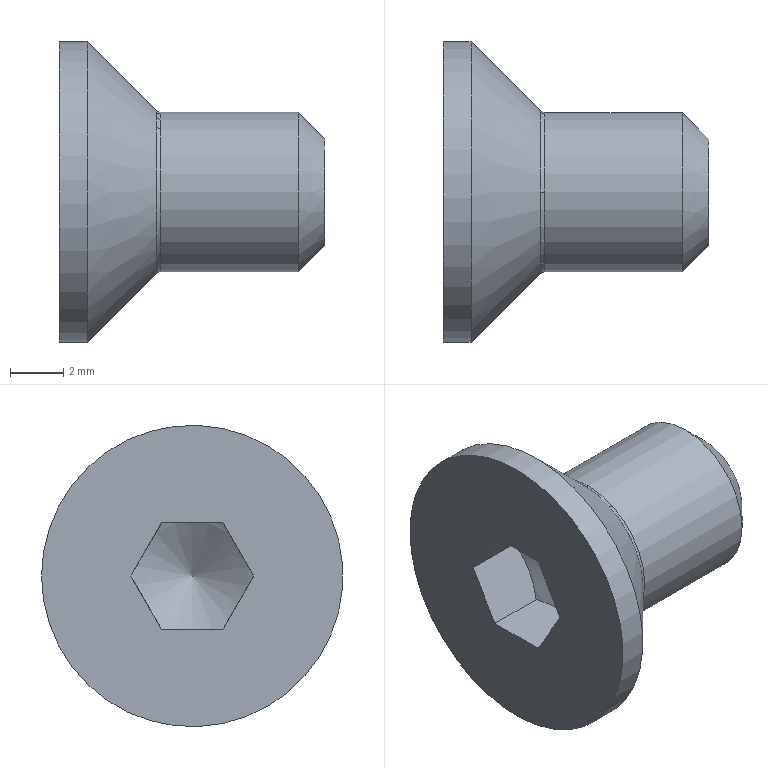Part | STEP file | Винт с потайной головкой и шестигранным углублением под ключ ГОСТ Р ИСО 10642 - М6 x 10 - 8.8 | 1 solid | 15 faces | box 10 x 11.34 x 11.34 mm | volume 400.146 mm3 | plane 8 | cone 3 | cylinder 2 | torus 2 | commonest cylinder face diameters 6 x1 11.34 x1
STEP:
#1=CARTESIAN_POINT('',(0.,5.67,0.));
#2=VERTEX_POINT('',#1);
#3=CARTESIAN_POINT('',(0.,0.,0.));
#4=DIRECTION('',(1.,0.,0.));
#5=DIRECTION('',(0.,1.,0.));
#6=AXIS2_PLACEMENT_3D('',#3,#4,#5);
#7=CIRCLE('',#6,5.67);
#8=EDGE_CURVE('',#2,#2,#7,.T.);
#9=ORIENTED_EDGE('',*,*,#8,.F.);
#10=EDGE_LOOP('',(#9));
#11=FACE_BOUND('',#10,.T.);
#12=CARTESIAN_POINT('',(0.,-1.155,2.));
#13=VERTEX_POINT('',#12);
#14=CARTESIAN_POINT('',(0.,-2.309,0.));
#15=VERTEX_POINT('',#14);
#16=CARTESIAN_POINT('',(0.,-1.155,2.));
#17=DIRECTION('',(0.,-0.5,-0.866));
#18=VECTOR('',#17,1.);
#19=LINE('',#16,#18);
#20=EDGE_CURVE('',#13,#15,#19,.T.);
#21=ORIENTED_EDGE('',*,*,#20,.T.);
#22=CARTESIAN_POINT('',(0.,-1.155,-2.));
#23=VERTEX_POINT('',#22);
#24=CARTESIAN_POINT('',(0.,-2.309,0.));
#25=DIRECTION('',(0.,0.5,-0.866));
#26=VECTOR('',#25,1.);
#27=LINE('',#24,#26);
#28=EDGE_CURVE('',#15,#23,#27,.T.);
#29=ORIENTED_EDGE('',*,*,#28,.T.);
#30=CARTESIAN_POINT('',(0.,1.155,-2.));
#31=VERTEX_POINT('',#30);
#32=CARTESIAN_POINT('',(0.,-1.155,-2.));
#33=DIRECTION('',(0.,1.,0.));
#34=VECTOR('',#33,1.);
#35=LINE('',#32,#34);
#36=EDGE_CURVE('',#23,#31,#35,.T.);
#37=ORIENTED_EDGE('',*,*,#36,.T.);
#38=CARTESIAN_POINT('',(0.,2.309,0.));
#39=VERTEX_POINT('',#38);
#40=CARTESIAN_POINT('',(0.,1.155,-2.));
#41=DIRECTION('',(0.,0.5,0.866));
#42=VECTOR('',#41,1.);
#43=LINE('',#40,#42);
#44=EDGE_CURVE('',#31,#39,#43,.T.);
#45=ORIENTED_EDGE('',*,*,#44,.T.);
#46=CARTESIAN_POINT('',(0.,1.155,2.));
#47=VERTEX_POINT('',#46);
#48=CARTESIAN_POINT('',(0.,2.309,0.));
#49=DIRECTION('',(0.,-0.5,0.866));
#50=VECTOR('',#49,1.);
#51=LINE('',#48,#50);
#52=EDGE_CURVE('',#39,#47,#51,.T.);
#53=ORIENTED_EDGE('',*,*,#52,.T.);
#54=CARTESIAN_POINT('',(0.,1.155,2.));
#55=DIRECTION('',(0.,-1.,0.));
#56=VECTOR('',#55,1.);
#57=LINE('',#54,#56);
#58=EDGE_CURVE('',#47,#13,#57,.T.);
#59=ORIENTED_EDGE('',*,*,#58,.T.);
#60=EDGE_LOOP('',(#21,#29,#37,#45,#53,#59));
#61=FACE_BOUND('',#60,.T.);
#62=CARTESIAN_POINT('',(0.,0.,0.));
#63=DIRECTION('',(1.,0.,0.));
#64=DIRECTION('',(0.,0.,1.));
#65=AXIS2_PLACEMENT_3D('',#62,#63,#64);
#66=PLANE('',#65);
#67=ADVANCED_FACE('',(#11,#61),#66,.F.);
#68=CARTESIAN_POINT('',(2.2,1.155,2.));
#69=VERTEX_POINT('',#68);
#70=CARTESIAN_POINT('',(2.379,0.,2.));
#71=VERTEX_POINT('',#70);
#72=CARTESIAN_POINT('',(2.379,0.,2.));
#73=CARTESIAN_POINT('',(2.379,0.03993,2.));
#74=CARTESIAN_POINT('',(2.378,0.09305,2.));
#75=CARTESIAN_POINT('',(2.374,0.1977,2.));
#76=CARTESIAN_POINT('',(2.367,0.2984,2.));
#77=CARTESIAN_POINT('',(2.356,0.3998,2.));
#78=CARTESIAN_POINT('',(2.342,0.5139,2.));
#79=CARTESIAN_POINT('',(2.325,0.6191,2.));
#80=CARTESIAN_POINT('',(2.301,0.7452,2.));
#81=CARTESIAN_POINT('',(2.279,0.8524,2.));
#82=CARTESIAN_POINT('',(2.256,0.9483,2.));
#83=CARTESIAN_POINT('',(2.232,1.04,2.));
#84=CARTESIAN_POINT('',(2.216,1.1,2.));
#85=CARTESIAN_POINT('',(2.203,1.143,2.));
#86=CARTESIAN_POINT('',(2.2,1.155,2.));
#87=B_SPLINE_CURVE_WITH_KNOTS('',3,(#72,#73,#74,#75,#76,#77,#78,#79,#80,#81,#82,#83,#84,#85,#86),.UNSPECIFIED.,.F.,.F.,(4,1,1,1,1,1,1,1,1,1,1,1,4),(0.,0.1021,0.1359,0.2681,0.3604,0.3966,0.5625,0.6326,0.7252,0.8429,0.8848,0.9686,1.),.UNSPECIFIED.);
#88=EDGE_CURVE('',#69,#71,#87,.F.);
#89=ORIENTED_EDGE('',*,*,#88,.F.);
#90=CARTESIAN_POINT('',(2.2,2.309,0.));
#91=VERTEX_POINT('',#90);
#92=CARTESIAN_POINT('',(2.2,1.155,2.));
#93=CARTESIAN_POINT('',(2.204,1.162,1.987));
#94=CARTESIAN_POINT('',(2.212,1.176,1.962));
#95=CARTESIAN_POINT('',(2.225,1.198,1.924));
#96=CARTESIAN_POINT('',(2.236,1.22,1.886));
#97=CARTESIAN_POINT('',(2.248,1.242,1.848));
#98=CARTESIAN_POINT('',(2.259,1.264,1.81));
#99=CARTESIAN_POINT('',(2.269,1.287,1.771));
#100=CARTESIAN_POINT('',(2.28,1.309,1.733));
#101=CARTESIAN_POINT('',(2.29,1.332,1.694));
#102=CARTESIAN_POINT('',(2.3,1.355,1.652));
#103=CARTESIAN_POINT('',(2.31,1.381,1.607));
#104=CARTESIAN_POINT('',(2.322,1.415,1.549));
#105=CARTESIAN_POINT('',(2.337,1.46,1.472));
#106=CARTESIAN_POINT('',(2.352,1.514,1.378));
#107=CARTESIAN_POINT('',(2.364,1.568,1.283));
#108=CARTESIAN_POINT('',(2.371,1.614,1.205));
#109=CARTESIAN_POINT('',(2.375,1.65,1.143));
#110=CARTESIAN_POINT('',(2.377,1.681,1.088));
#111=CARTESIAN_POINT('',(2.378,1.709,1.04));
#112=CARTESIAN_POINT('',(2.379,1.731,1.002));
#113=CARTESIAN_POINT('',(2.379,1.753,0.9644));
#114=CARTESIAN_POINT('',(2.378,1.78,0.9178));
#115=CARTESIAN_POINT('',(2.375,1.813,0.8602));
#116=CARTESIAN_POINT('',(2.371,1.846,0.8026));
#117=CARTESIAN_POINT('',(2.366,1.879,0.7449));
#118=CARTESIAN_POINT('',(2.36,1.913,0.6872));
#119=CARTESIAN_POINT('',(2.353,1.946,0.6295));
#120=CARTESIAN_POINT('',(2.344,1.979,0.5718));
#121=CARTESIAN_POINT('',(2.334,2.013,0.5142));
#122=CARTESIAN_POINT('',(2.323,2.046,0.4566));
#123=CARTESIAN_POINT('',(2.311,2.079,0.3992));
#124=CARTESIAN_POINT('',(2.298,2.112,0.3418));
#125=CARTESIAN_POINT('',(2.284,2.145,0.2846));
#126=CARTESIAN_POINT('',(2.269,2.178,0.2274));
#127=CARTESIAN_POINT('',(2.253,2.211,0.1704));
#128=CARTESIAN_POINT('',(2.236,2.244,0.1134));
#129=CARTESIAN_POINT('',(2.219,2.277,0.05661));
#130=CARTESIAN_POINT('',(2.206,2.299,0.01885));
#131=CARTESIAN_POINT('',(2.2,2.309,0.));
#132=B_SPLINE_CURVE_WITH_KNOTS('',3,(#92,#93,#94,#95,#96,#97,#98,#99,#100,#101,#102,#103,#104,#105,#106,#107,#108,#109,#110,#111,#112,#113,#114,#115,#116,#117,#118,#119,#120,#121,#122,#123,#124,#125,#126,#127,#128,#129,#130,#131),.UNSPECIFIED.,.F.,.F.,(4,1,1,1,1,1,1,1,1,1,1,1,1,1,1,1,1,1,1,1,1,1,1,1,1,1,1,1,1,1,1,1,1,1,1,1,1,4),(0.,0.01933,0.03868,0.05804,0.07746,0.0969,0.1164,0.136,0.1557,0.1754,0.1981,0.2236,0.2627,0.3137,0.3641,0.403,0.4296,0.4566,0.4843,0.5,0.5121,0.5404,0.5688,0.5973,0.6258,0.6543,0.6829,0.7116,0.7402,0.7689,0.7977,0.8264,0.8552,0.8841,0.913,0.9419,0.9709,1.),.UNSPECIFIED.);
#133=EDGE_CURVE('',#91,#69,#132,.F.);
#134=ORIENTED_EDGE('',*,*,#133,.F.);
#135=CARTESIAN_POINT('',(2.2,1.155,-2.));
#136=VERTEX_POINT('',#135);
#137=CARTESIAN_POINT('',(2.2,2.309,0.));
#138=CARTESIAN_POINT('',(2.204,2.302,-0.01256));
#139=CARTESIAN_POINT('',(2.212,2.288,-0.03772));
#140=CARTESIAN_POINT('',(2.225,2.266,-0.07557));
#141=CARTESIAN_POINT('',(2.236,2.244,-0.1136));
#142=CARTESIAN_POINT('',(2.248,2.222,-0.1517));
#143=CARTESIAN_POINT('',(2.259,2.2,-0.1901));
#144=CARTESIAN_POINT('',(2.269,2.177,-0.2286));
#145=CARTESIAN_POINT('',(2.28,2.155,-0.2674));
#146=CARTESIAN_POINT('',(2.29,2.132,-0.3065));
#147=CARTESIAN_POINT('',(2.3,2.109,-0.3476));
#148=CARTESIAN_POINT('',(2.31,2.083,-0.3926));
#149=CARTESIAN_POINT('',(2.322,2.049,-0.4507));
#150=CARTESIAN_POINT('',(2.337,2.005,-0.528));
#151=CARTESIAN_POINT('',(2.352,1.95,-0.6222));
#152=CARTESIAN_POINT('',(2.364,1.896,-0.7166));
#153=CARTESIAN_POINT('',(2.371,1.85,-0.7949));
#154=CARTESIAN_POINT('',(2.375,1.814,-0.8574));
#155=CARTESIAN_POINT('',(2.377,1.783,-0.9124));
#156=CARTESIAN_POINT('',(2.378,1.755,-0.96));
#157=CARTESIAN_POINT('',(2.379,1.733,-0.9976));
#158=CARTESIAN_POINT('',(2.379,1.711,-1.036));
#159=CARTESIAN_POINT('',(2.378,1.685,-1.082));
#160=CARTESIAN_POINT('',(2.375,1.651,-1.14));
#161=CARTESIAN_POINT('',(2.371,1.618,-1.197));
#162=CARTESIAN_POINT('',(2.366,1.585,-1.255));
#163=CARTESIAN_POINT('',(2.36,1.551,-1.313));
#164=CARTESIAN_POINT('',(2.353,1.518,-1.371));
#165=CARTESIAN_POINT('',(2.344,1.485,-1.428));
#166=CARTESIAN_POINT('',(2.334,1.452,-1.486));
#167=CARTESIAN_POINT('',(2.323,1.418,-1.543));
#168=CARTESIAN_POINT('',(2.311,1.385,-1.601));
#169=CARTESIAN_POINT('',(2.298,1.352,-1.658));
#170=CARTESIAN_POINT('',(2.284,1.319,-1.715));
#171=CARTESIAN_POINT('',(2.269,1.286,-1.773));
#172=CARTESIAN_POINT('',(2.253,1.253,-1.83));
#173=CARTESIAN_POINT('',(2.236,1.22,-1.887));
#174=CARTESIAN_POINT('',(2.219,1.187,-1.943));
#175=CARTESIAN_POINT('',(2.206,1.166,-1.981));
#176=CARTESIAN_POINT('',(2.2,1.155,-2.));
#177=B_SPLINE_CURVE_WITH_KNOTS('',3,(#137,#138,#139,#140,#141,#142,#143,#144,#145,#146,#147,#148,#149,#150,#151,#152,#153,#154,#155,#156,#157,#158,#159,#160,#161,#162,#163,#164,#165,#166,#167,#168,#169,#170,#171,#172,#173,#174,#175,#176),.UNSPECIFIED.,.F.,.F.,(4,1,1,1,1,1,1,1,1,1,1,1,1,1,1,1,1,1,1,1,1,1,1,1,1,1,1,1,1,1,1,1,1,1,1,1,1,4),(0.,0.01933,0.03868,0.05804,0.07746,0.0969,0.1164,0.136,0.1557,0.1754,0.1981,0.2236,0.2627,0.3137,0.3641,0.403,0.4296,0.4566,0.4843,0.5,0.5121,0.5404,0.5688,0.5973,0.6258,0.6543,0.6829,0.7116,0.7402,0.7689,0.7977,0.8264,0.8552,0.8841,0.913,0.9419,0.9709,1.),.UNSPECIFIED.);
#178=EDGE_CURVE('',#136,#91,#177,.F.);
#179=ORIENTED_EDGE('',*,*,#178,.F.);
#180=CARTESIAN_POINT('',(2.2,-1.155,-2.));
#181=VERTEX_POINT('',#180);
#182=CARTESIAN_POINT('',(2.2,1.155,-2.));
#183=CARTESIAN_POINT('',(2.204,1.14,-2.));
#184=CARTESIAN_POINT('',(2.212,1.111,-2.));
#185=CARTESIAN_POINT('',(2.225,1.067,-2.));
#186=CARTESIAN_POINT('',(2.236,1.026,-2.));
#187=CARTESIAN_POINT('',(2.243,0.9963,-2.));
#188=CARTESIAN_POINT('',(2.251,0.9668,-2.));
#189=CARTESIAN_POINT('',(2.259,0.9352,-2.));
#190=CARTESIAN_POINT('',(2.269,0.8907,-2.));
#191=CARTESIAN_POINT('',(2.28,0.8459,-2.));
#192=CARTESIAN_POINT('',(2.29,0.8008,-2.));
#193=CARTESIAN_POINT('',(2.3,0.7534,-2.));
#194=CARTESIAN_POINT('',(2.31,0.7013,-2.));
#195=CARTESIAN_POINT('',(2.317,0.6639,-2.));
#196=CARTESIAN_POINT('',(2.326,0.6142,-2.));
#197=CARTESIAN_POINT('',(2.337,0.5447,-2.));
#198=CARTESIAN_POINT('',(2.349,0.4569,-2.));
#199=CARTESIAN_POINT('',(2.358,0.3781,-2.));
#200=CARTESIAN_POINT('',(2.365,0.3087,-2.));
#201=CARTESIAN_POINT('',(2.37,0.2457,-2.));
#202=CARTESIAN_POINT('',(2.373,0.1946,-2.));
#203=CARTESIAN_POINT('',(2.375,0.1527,-2.));
#204=CARTESIAN_POINT('',(2.377,0.1011,-2.));
#205=CARTESIAN_POINT('',(2.378,0.04616,-2.));
#206=CARTESIAN_POINT('',(2.379,0.002789,-2.));
#207=CARTESIAN_POINT('',(2.379,-0.04112,-2.));
#208=CARTESIAN_POINT('',(2.378,-0.07585,-2.));
#209=CARTESIAN_POINT('',(2.377,-0.1201,-2.));
#210=CARTESIAN_POINT('',(2.375,-0.1645,-2.));
#211=CARTESIAN_POINT('',(2.371,-0.228,-2.));
#212=CARTESIAN_POINT('',(2.366,-0.2946,-2.));
#213=CARTESIAN_POINT('',(2.361,-0.3498,-2.));
#214=CARTESIAN_POINT('',(2.356,-0.3942,-2.));
#215=CARTESIAN_POINT('',(2.351,-0.4386,-2.));
#216=CARTESIAN_POINT('',(2.344,-0.4944,-2.));
#217=CARTESIAN_POINT('',(2.335,-0.5545,-2.));
#218=CARTESIAN_POINT('',(2.328,-0.5988,-2.));
#219=CARTESIAN_POINT('',(2.32,-0.6431,-2.));
#220=CARTESIAN_POINT('',(2.311,-0.6938,-2.));
#221=CARTESIAN_POINT('',(2.298,-0.76,-2.));
#222=CARTESIAN_POINT('',(2.285,-0.8199,-2.));
#223=CARTESIAN_POINT('',(2.276,-0.8639,-2.));
#224=CARTESIAN_POINT('',(2.265,-0.9079,-2.));
#225=CARTESIAN_POINT('',(2.253,-0.958,-2.));
#226=CARTESIAN_POINT('',(2.237,-1.023,-2.));
#227=CARTESIAN_POINT('',(2.225,-1.066,-2.));
#228=CARTESIAN_POINT('',(2.213,-1.11,-2.));
#229=CARTESIAN_POINT('',(2.206,-1.133,-2.));
#230=CARTESIAN_POINT('',(2.2,-1.155,-2.));
#231=B_SPLINE_CURVE_WITH_KNOTS('',3,(#182,#183,#184,#185,#186,#187,#188,#189,#190,#191,#192,#193,#194,#195,#196,#197,#198,#199,#200,#201,#202,#203,#204,#205,#206,#207,#208,#209,#210,#211,#212,#213,#214,#215,#216,#217,#218,#219,#220,#221,#222,#223,#224,#225,#226,#227,#228,#229,#230),.UNSPECIFIED.,.F.,.F.,(4,1,1,1,1,1,1,1,1,1,1,1,1,1,1,1,1,1,1,1,1,1,1,1,1,1,1,1,1,1,1,1,1,1,1,1,1,1,1,1,1,1,1,1,1,1,4),(0.,0.01933,0.03868,0.05804,0.07472,0.07746,0.0969,0.1164,0.136,0.1557,0.1754,0.1981,0.2236,0.2241,0.2627,0.3137,0.3375,0.3641,0.403,0.4183,0.4296,0.4566,0.4843,0.5,0.5121,0.5404,0.5444,0.5688,0.5973,0.6258,0.6543,0.6683,0.6829,0.7116,0.7402,0.7605,0.7689,0.7977,0.8264,0.8552,0.876,0.8841,0.913,0.9419,0.9694,0.9709,1.),.UNSPECIFIED.);
#232=EDGE_CURVE('',#181,#136,#231,.F.);
#233=ORIENTED_EDGE('',*,*,#232,.F.);
#234=CARTESIAN_POINT('',(2.2,-2.309,0.));
#235=VERTEX_POINT('',#234);
#236=CARTESIAN_POINT('',(2.2,-1.155,-2.));
#237=CARTESIAN_POINT('',(2.204,-1.162,-1.987));
#238=CARTESIAN_POINT('',(2.212,-1.176,-1.962));
#239=CARTESIAN_POINT('',(2.225,-1.198,-1.924));
#240=CARTESIAN_POINT('',(2.236,-1.22,-1.886));
#241=CARTESIAN_POINT('',(2.248,-1.242,-1.848));
#242=CARTESIAN_POINT('',(2.259,-1.264,-1.81));
#243=CARTESIAN_POINT('',(2.269,-1.287,-1.771));
#244=CARTESIAN_POINT('',(2.28,-1.309,-1.733));
#245=CARTESIAN_POINT('',(2.29,-1.332,-1.694));
#246=CARTESIAN_POINT('',(2.3,-1.355,-1.652));
#247=CARTESIAN_POINT('',(2.31,-1.381,-1.607));
#248=CARTESIAN_POINT('',(2.322,-1.415,-1.549));
#249=CARTESIAN_POINT('',(2.337,-1.459,-1.472));
#250=CARTESIAN_POINT('',(2.352,-1.514,-1.378));
#251=CARTESIAN_POINT('',(2.364,-1.568,-1.284));
#252=CARTESIAN_POINT('',(2.371,-1.613,-1.206));
#253=CARTESIAN_POINT('',(2.375,-1.649,-1.144));
#254=CARTESIAN_POINT('',(2.377,-1.681,-1.089));
#255=CARTESIAN_POINT('',(2.378,-1.708,-1.041));
#256=CARTESIAN_POINT('',(2.379,-1.73,-1.003));
#257=CARTESIAN_POINT('',(2.379,-1.752,-0.9655));
#258=CARTESIAN_POINT('',(2.378,-1.779,-0.9195));
#259=CARTESIAN_POINT('',(2.375,-1.812,-0.862));
#260=CARTESIAN_POINT('',(2.372,-1.845,-0.8045));
#261=CARTESIAN_POINT('',(2.367,-1.878,-0.7468));
#262=CARTESIAN_POINT('',(2.36,-1.912,-0.6892));
#263=CARTESIAN_POINT('',(2.353,-1.945,-0.6314));
#264=CARTESIAN_POINT('',(2.344,-1.978,-0.5737));
#265=CARTESIAN_POINT('',(2.335,-2.011,-0.516));
#266=CARTESIAN_POINT('',(2.324,-2.045,-0.4583));
#267=CARTESIAN_POINT('',(2.312,-2.078,-0.4007));
#268=CARTESIAN_POINT('',(2.299,-2.111,-0.3432));
#269=CARTESIAN_POINT('',(2.284,-2.144,-0.2857));
#270=CARTESIAN_POINT('',(2.269,-2.178,-0.2284));
#271=CARTESIAN_POINT('',(2.253,-2.211,-0.1711));
#272=CARTESIAN_POINT('',(2.236,-2.244,-0.1139));
#273=CARTESIAN_POINT('',(2.219,-2.277,-0.05687));
#274=CARTESIAN_POINT('',(2.206,-2.298,-0.01894));
#275=CARTESIAN_POINT('',(2.2,-2.309,0.));
#276=B_SPLINE_CURVE_WITH_KNOTS('',3,(#236,#237,#238,#239,#240,#241,#242,#243,#244,#245,#246,#247,#248,#249,#250,#251,#252,#253,#254,#255,#256,#257,#258,#259,#260,#261,#262,#263,#264,#265,#266,#267,#268,#269,#270,#271,#272,#273,#274,#275),.UNSPECIFIED.,.F.,.F.,(4,1,1,1,1,1,1,1,1,1,1,1,1,1,1,1,1,1,1,1,1,1,1,1,1,1,1,1,1,1,1,1,1,1,1,1,1,4),(0.,0.01933,0.03868,0.05804,0.07746,0.0969,0.1164,0.136,0.1557,0.1754,0.198,0.2236,0.2626,0.3135,0.3638,0.4026,0.4291,0.456,0.4836,0.5,0.5114,0.5396,0.5679,0.5963,0.6248,0.6533,0.6819,0.7106,0.7393,0.7681,0.7969,0.8257,0.8546,0.8836,0.9126,0.9417,0.9708,1.),.UNSPECIFIED.);
#277=EDGE_CURVE('',#235,#181,#276,.F.);
#278=ORIENTED_EDGE('',*,*,#277,.F.);
#279=CARTESIAN_POINT('',(2.2,-1.155,2.));
#280=VERTEX_POINT('',#279);
#281=CARTESIAN_POINT('',(2.2,-2.309,0.));
#282=CARTESIAN_POINT('',(2.204,-2.302,0.01256));
#283=CARTESIAN_POINT('',(2.212,-2.288,0.03772));
#284=CARTESIAN_POINT('',(2.225,-2.266,0.07557));
#285=CARTESIAN_POINT('',(2.236,-2.244,0.1136));
#286=CARTESIAN_POINT('',(2.248,-2.222,0.1517));
#287=CARTESIAN_POINT('',(2.259,-2.2,0.1901));
#288=CARTESIAN_POINT('',(2.269,-2.177,0.2286));
#289=CARTESIAN_POINT('',(2.28,-2.155,0.2674));
#290=CARTESIAN_POINT('',(2.29,-2.132,0.3065));
#291=CARTESIAN_POINT('',(2.3,-2.109,0.3476));
#292=CARTESIAN_POINT('',(2.31,-2.083,0.3926));
#293=CARTESIAN_POINT('',(2.322,-2.049,0.4507));
#294=CARTESIAN_POINT('',(2.337,-2.005,0.528));
#295=CARTESIAN_POINT('',(2.352,-1.95,0.6222));
#296=CARTESIAN_POINT('',(2.364,-1.896,0.7166));
#297=CARTESIAN_POINT('',(2.371,-1.85,0.7949));
#298=CARTESIAN_POINT('',(2.375,-1.814,0.8574));
#299=CARTESIAN_POINT('',(2.377,-1.783,0.9124));
#300=CARTESIAN_POINT('',(2.378,-1.755,0.96));
#301=CARTESIAN_POINT('',(2.379,-1.733,0.9976));
#302=CARTESIAN_POINT('',(2.379,-1.711,1.036));
#303=CARTESIAN_POINT('',(2.378,-1.685,1.082));
#304=CARTESIAN_POINT('',(2.375,-1.651,1.14));
#305=CARTESIAN_POINT('',(2.371,-1.618,1.197));
#306=CARTESIAN_POINT('',(2.366,-1.585,1.255));
#307=CARTESIAN_POINT('',(2.36,-1.551,1.313));
#308=CARTESIAN_POINT('',(2.353,-1.518,1.371));
#309=CARTESIAN_POINT('',(2.344,-1.485,1.428));
#310=CARTESIAN_POINT('',(2.334,-1.452,1.486));
#311=CARTESIAN_POINT('',(2.323,-1.418,1.543));
#312=CARTESIAN_POINT('',(2.311,-1.385,1.601));
#313=CARTESIAN_POINT('',(2.298,-1.352,1.658));
#314=CARTESIAN_POINT('',(2.284,-1.319,1.715));
#315=CARTESIAN_POINT('',(2.269,-1.286,1.773));
#316=CARTESIAN_POINT('',(2.253,-1.253,1.83));
#317=CARTESIAN_POINT('',(2.236,-1.22,1.887));
#318=CARTESIAN_POINT('',(2.219,-1.187,1.943));
#319=CARTESIAN_POINT('',(2.206,-1.166,1.981));
#320=CARTESIAN_POINT('',(2.2,-1.155,2.));
#321=B_SPLINE_CURVE_WITH_KNOTS('',3,(#281,#282,#283,#284,#285,#286,#287,#288,#289,#290,#291,#292,#293,#294,#295,#296,#297,#298,#299,#300,#301,#302,#303,#304,#305,#306,#307,#308,#309,#310,#311,#312,#313,#314,#315,#316,#317,#318,#319,#320),.UNSPECIFIED.,.F.,.F.,(4,1,1,1,1,1,1,1,1,1,1,1,1,1,1,1,1,1,1,1,1,1,1,1,1,1,1,1,1,1,1,1,1,1,1,1,1,4),(0.,0.01933,0.03868,0.05804,0.07746,0.0969,0.1164,0.136,0.1557,0.1754,0.1981,0.2236,0.2627,0.3137,0.3641,0.403,0.4296,0.4566,0.4843,0.5,0.5121,0.5404,0.5688,0.5973,0.6258,0.6543,0.6829,0.7116,0.7402,0.7689,0.7977,0.8264,0.8552,0.8841,0.913,0.9419,0.9709,1.),.UNSPECIFIED.);
#322=EDGE_CURVE('',#280,#235,#321,.F.);
#323=ORIENTED_EDGE('',*,*,#322,.F.);
#324=CARTESIAN_POINT('',(2.2,-1.155,2.));
#325=CARTESIAN_POINT('',(2.208,-1.128,2.));
#326=CARTESIAN_POINT('',(2.224,-1.07,2.));
#327=CARTESIAN_POINT('',(2.246,-0.9856,2.));
#328=CARTESIAN_POINT('',(2.27,-0.8898,2.));
#329=CARTESIAN_POINT('',(2.291,-0.7956,2.));
#330=CARTESIAN_POINT('',(2.311,-0.698,2.));
#331=CARTESIAN_POINT('',(2.33,-0.5909,2.));
#332=CARTESIAN_POINT('',(2.342,-0.5072,2.));
#333=CARTESIAN_POINT('',(2.355,-0.4061,2.));
#334=CARTESIAN_POINT('',(2.365,-0.3138,2.));
#335=CARTESIAN_POINT('',(2.372,-0.2169,2.));
#336=CARTESIAN_POINT('',(2.377,-0.121,2.));
#337=CARTESIAN_POINT('',(2.379,-0.05776,2.));
#338=CARTESIAN_POINT('',(2.379,-0.005712,2.));
#339=CARTESIAN_POINT('',(2.379,-0.000000001,2.));
#340=B_SPLINE_CURVE_WITH_KNOTS('',3,(#324,#325,#326,#327,#328,#329,#330,#331,#332,#333,#334,#335,#336,#337,#338,#339),.UNSPECIFIED.,.F.,.F.,(4,1,1,1,1,1,1,1,1,1,1,1,1,4),(0.,0.07,0.1546,0.224,0.3223,0.4019,0.4787,0.6006,0.6184,0.7397,0.8381,0.8669,0.9854,1.),.UNSPECIFIED.);
#341=EDGE_CURVE('',#71,#280,#340,.F.);
#342=ORIENTED_EDGE('',*,*,#341,.F.);
#343=EDGE_LOOP('',(#89,#134,#179,#233,#278,#323,#342));
#344=FACE_BOUND('',#343,.T.);
#345=CARTESIAN_POINT('',(2.867,0.,0.));
#346=DIRECTION('',(-1.,0.,0.));
#347=DIRECTION('',(0.,0.,-1.));
#348=AXIS2_PLACEMENT_3D('',#345,#346,#347);
#349=CONICAL_SURFACE('',#348,1.155,1.047);
#350=ADVANCED_FACE('',(#344),#349,.F.);
#351=ORIENTED_EDGE('',*,*,#341,.T.);
#352=CARTESIAN_POINT('',(0.,-1.155,2.));
#353=DIRECTION('',(1.,0.,0.));
#354=VECTOR('',#353,1.);
#355=LINE('',#352,#354);
#356=EDGE_CURVE('',#13,#280,#355,.T.);
#357=ORIENTED_EDGE('',*,*,#356,.F.);
#358=ORIENTED_EDGE('',*,*,#58,.F.);
#359=CARTESIAN_POINT('',(0.,1.155,2.));
#360=DIRECTION('',(1.,0.,0.));
#361=VECTOR('',#360,1.);
#362=LINE('',#359,#361);
#363=EDGE_CURVE('',#47,#69,#362,.T.);
#364=ORIENTED_EDGE('',*,*,#363,.T.);
#365=ORIENTED_EDGE('',*,*,#88,.T.);
#366=EDGE_LOOP('',(#351,#357,#358,#364,#365));
#367=FACE_BOUND('',#366,.T.);
#368=CARTESIAN_POINT('',(0.,1.155,2.));
#369=DIRECTION('',(0.,0.,1.));
#370=DIRECTION('',(0.,-1.,0.));
#371=AXIS2_PLACEMENT_3D('',#368,#369,#370);
#372=PLANE('',#371);
#373=ADVANCED_FACE('',(#367),#372,.F.);
#374=ORIENTED_EDGE('',*,*,#133,.T.);
#375=ORIENTED_EDGE('',*,*,#363,.F.);
#376=ORIENTED_EDGE('',*,*,#52,.F.);
#377=CARTESIAN_POINT('',(0.,2.309,0.));
#378=DIRECTION('',(1.,0.,0.));
#379=VECTOR('',#378,1.);
#380=LINE('',#377,#379);
#381=EDGE_CURVE('',#39,#91,#380,.T.);
#382=ORIENTED_EDGE('',*,*,#381,.T.);
#383=EDGE_LOOP('',(#374,#375,#376,#382));
#384=FACE_BOUND('',#383,.T.);
#385=CARTESIAN_POINT('',(0.,2.309,0.));
#386=DIRECTION('',(0.,0.866,0.5));
#387=DIRECTION('',(0.,-0.5,0.866));
#388=AXIS2_PLACEMENT_3D('',#385,#386,#387);
#389=PLANE('',#388);
#390=ADVANCED_FACE('',(#384),#389,.F.);
#391=ORIENTED_EDGE('',*,*,#178,.T.);
#392=ORIENTED_EDGE('',*,*,#381,.F.);
#393=ORIENTED_EDGE('',*,*,#44,.F.);
#394=CARTESIAN_POINT('',(0.,1.155,-2.));
#395=DIRECTION('',(1.,0.,0.));
#396=VECTOR('',#395,1.);
#397=LINE('',#394,#396);
#398=EDGE_CURVE('',#31,#136,#397,.T.);
#399=ORIENTED_EDGE('',*,*,#398,.T.);
#400=EDGE_LOOP('',(#391,#392,#393,#399));
#401=FACE_BOUND('',#400,.T.);
#402=CARTESIAN_POINT('',(0.,1.155,-2.));
#403=DIRECTION('',(0.,0.866,-0.5));
#404=DIRECTION('',(0.,0.5,0.866));
#405=AXIS2_PLACEMENT_3D('',#402,#403,#404);
#406=PLANE('',#405);
#407=ADVANCED_FACE('',(#401),#406,.F.);
#408=ORIENTED_EDGE('',*,*,#232,.T.);
#409=ORIENTED_EDGE('',*,*,#398,.F.);
#410=ORIENTED_EDGE('',*,*,#36,.F.);
#411=CARTESIAN_POINT('',(0.,-1.155,-2.));
#412=DIRECTION('',(1.,0.,0.));
#413=VECTOR('',#412,1.);
#414=LINE('',#411,#413);
#415=EDGE_CURVE('',#23,#181,#414,.T.);
#416=ORIENTED_EDGE('',*,*,#415,.T.);
#417=EDGE_LOOP('',(#408,#409,#410,#416));
#418=FACE_BOUND('',#417,.T.);
#419=CARTESIAN_POINT('',(0.,-1.155,-2.));
#420=DIRECTION('',(0.,0.,-1.));
#421=DIRECTION('',(0.,1.,0.));
#422=AXIS2_PLACEMENT_3D('',#419,#420,#421);
#423=PLANE('',#422);
#424=ADVANCED_FACE('',(#418),#423,.F.);
#425=ORIENTED_EDGE('',*,*,#277,.T.);
#426=ORIENTED_EDGE('',*,*,#415,.F.);
#427=ORIENTED_EDGE('',*,*,#28,.F.);
#428=CARTESIAN_POINT('',(0.,-2.309,0.));
#429=DIRECTION('',(1.,0.,0.));
#430=VECTOR('',#429,1.);
#431=LINE('',#428,#430);
#432=EDGE_CURVE('',#15,#235,#431,.T.);
#433=ORIENTED_EDGE('',*,*,#432,.T.);
#434=EDGE_LOOP('',(#425,#426,#427,#433));
#435=FACE_BOUND('',#434,.T.);
#436=CARTESIAN_POINT('',(0.,-2.309,0.));
#437=DIRECTION('',(0.,-0.866,-0.5));
#438=DIRECTION('',(0.,0.5,-0.866));
#439=AXIS2_PLACEMENT_3D('',#436,#437,#438);
#440=PLANE('',#439);
#441=ADVANCED_FACE('',(#435),#440,.F.);
#442=ORIENTED_EDGE('',*,*,#322,.T.);
#443=ORIENTED_EDGE('',*,*,#432,.F.);
#444=ORIENTED_EDGE('',*,*,#20,.F.);
#445=ORIENTED_EDGE('',*,*,#356,.T.);
#446=EDGE_LOOP('',(#442,#443,#444,#445));
#447=FACE_BOUND('',#446,.T.);
#448=CARTESIAN_POINT('',(0.,-1.155,2.));
#449=DIRECTION('',(0.,-0.866,0.5));
#450=DIRECTION('',(0.,-0.5,-0.866));
#451=AXIS2_PLACEMENT_3D('',#448,#449,#450);
#452=PLANE('',#451);
#453=ADVANCED_FACE('',(#447),#452,.F.);
#454=CARTESIAN_POINT('',(1.05,5.67,0.));
#455=VERTEX_POINT('',#454);
#456=CARTESIAN_POINT('',(1.05,0.,0.));
#457=DIRECTION('',(1.,0.,0.));
#458=DIRECTION('',(0.,1.,0.));
#459=AXIS2_PLACEMENT_3D('',#456,#457,#458);
#460=CIRCLE('',#459,5.67);
#461=EDGE_CURVE('',#455,#455,#460,.T.);
#462=ORIENTED_EDGE('',*,*,#461,.F.);
#463=EDGE_LOOP('',(#462));
#464=FACE_OUTER_BOUND('',#463,.T.);
#465=ORIENTED_EDGE('',*,*,#8,.T.);
#466=EDGE_LOOP('',(#465));
#467=FACE_OUTER_BOUND('',#466,.T.);
#468=CARTESIAN_POINT('',(0.,0.,0.));
#469=DIRECTION('',(1.,0.,0.));
#470=DIRECTION('',(0.,1.,0.));
#471=AXIS2_PLACEMENT_3D('',#468,#469,#470);
#472=CYLINDRICAL_SURFACE('',#471,5.67);
#473=ADVANCED_FACE('',(#464,#467),#472,.T.);
#474=CARTESIAN_POINT('',(3.647,3.073,0.));
#475=VERTEX_POINT('',#474);
#476=CARTESIAN_POINT('',(3.647,0.,3.073));
#477=VERTEX_POINT('',#476);
#478=CARTESIAN_POINT('',(3.647,0.,0.));
#479=DIRECTION('',(1.,0.,0.));
#480=DIRECTION('',(0.,0.,1.));
#481=AXIS2_PLACEMENT_3D('',#478,#479,#480);
#482=CIRCLE('',#481,3.073);
#483=EDGE_CURVE('',#475,#477,#482,.F.);
#484=ORIENTED_EDGE('',*,*,#483,.T.);
#485=CARTESIAN_POINT('',(3.647,0.,0.));
#486=DIRECTION('',(1.,0.,0.));
#487=DIRECTION('',(0.,1.,0.));
#488=AXIS2_PLACEMENT_3D('',#485,#486,#487);
#489=CIRCLE('',#488,3.073);
#490=EDGE_CURVE('',#477,#475,#489,.F.);
#491=ORIENTED_EDGE('',*,*,#490,.T.);
#492=EDGE_LOOP('',(#484,#491));
#493=FACE_BOUND('',#492,.T.);
#494=ORIENTED_EDGE('',*,*,#461,.T.);
#495=EDGE_LOOP('',(#494));
#496=FACE_OUTER_BOUND('',#495,.T.);
#497=CARTESIAN_POINT('',(2.348,0.,0.));
#498=DIRECTION('',(-1.,0.,0.));
#499=DIRECTION('',(0.,-1.,0.));
#500=AXIS2_PLACEMENT_3D('',#497,#498,#499);
#501=CONICAL_SURFACE('',#500,4.372,0.7854);
#502=ADVANCED_FACE('',(#493,#496),#501,.T.);
#503=CARTESIAN_POINT('',(3.824,0.,3.));
#504=VERTEX_POINT('',#503);
#505=CARTESIAN_POINT('',(3.824,3.,0.));
#506=VERTEX_POINT('',#505);
#507=CARTESIAN_POINT('',(3.824,0.,0.));
#508=DIRECTION('',(1.,0.,0.));
#509=DIRECTION('',(0.,1.,0.));
#510=AXIS2_PLACEMENT_3D('',#507,#508,#509);
#511=CIRCLE('',#510,3.);
#512=EDGE_CURVE('',#504,#506,#511,.F.);
#513=ORIENTED_EDGE('',*,*,#512,.T.);
#514=CARTESIAN_POINT('',(3.824,3.25,0.));
#515=DIRECTION('',(0.,0.,-1.));
#516=DIRECTION('',(0.,-1.,0.));
#517=AXIS2_PLACEMENT_3D('',#514,#515,#516);
#518=CIRCLE('',#517,0.25);
#519=EDGE_CURVE('',#506,#475,#518,.T.);
#520=ORIENTED_EDGE('',*,*,#519,.T.);
#521=ORIENTED_EDGE('',*,*,#490,.F.);
#522=CARTESIAN_POINT('',(3.824,0.,3.25));
#523=DIRECTION('',(0.,1.,0.));
#524=DIRECTION('',(0.,0.,-1.));
#525=AXIS2_PLACEMENT_3D('',#522,#523,#524);
#526=CIRCLE('',#525,0.25);
#527=EDGE_CURVE('',#504,#477,#526,.T.);
#528=ORIENTED_EDGE('',*,*,#527,.F.);
#529=EDGE_LOOP('',(#513,#520,#521,#528));
#530=FACE_BOUND('',#529,.T.);
#531=CARTESIAN_POINT('',(3.824,0.,0.));
#532=DIRECTION('',(1.,0.,0.));
#533=DIRECTION('',(0.,0.9861,-0.1659));
#534=AXIS2_PLACEMENT_3D('',#531,#532,#533);
#535=TOROIDAL_SURFACE('',#534,3.25,0.25);
#536=ADVANCED_FACE('',(#530),#535,.F.);
#537=CARTESIAN_POINT('',(3.824,0.,0.));
#538=DIRECTION('',(1.,0.,0.));
#539=DIRECTION('',(0.,0.,1.));
#540=AXIS2_PLACEMENT_3D('',#537,#538,#539);
#541=CIRCLE('',#540,3.);
#542=EDGE_CURVE('',#506,#504,#541,.F.);
#543=ORIENTED_EDGE('',*,*,#542,.T.);
#544=ORIENTED_EDGE('',*,*,#527,.T.);
#545=ORIENTED_EDGE('',*,*,#483,.F.);
#546=ORIENTED_EDGE('',*,*,#519,.F.);
#547=EDGE_LOOP('',(#543,#544,#545,#546));
#548=FACE_BOUND('',#547,.T.);
#549=CARTESIAN_POINT('',(3.824,0.,0.));
#550=DIRECTION('',(1.,0.,0.));
#551=DIRECTION('',(0.,0.1659,0.9861));
#552=AXIS2_PLACEMENT_3D('',#549,#550,#551);
#553=TOROIDAL_SURFACE('',#552,3.25,0.25);
#554=ADVANCED_FACE('',(#548),#553,.F.);
#555=CARTESIAN_POINT('',(9.,0.,3.));
#556=VERTEX_POINT('',#555);
#557=CARTESIAN_POINT('',(9.,0.,0.));
#558=DIRECTION('',(1.,0.,0.));
#559=DIRECTION('',(0.,0.,1.));
#560=AXIS2_PLACEMENT_3D('',#557,#558,#559);
#561=CIRCLE('',#560,3.);
#562=EDGE_CURVE('',#556,#556,#561,.T.);
#563=ORIENTED_EDGE('',*,*,#562,.F.);
#564=EDGE_LOOP('',(#563));
#565=FACE_OUTER_BOUND('',#564,.T.);
#566=ORIENTED_EDGE('',*,*,#512,.F.);
#567=ORIENTED_EDGE('',*,*,#542,.F.);
#568=EDGE_LOOP('',(#566,#567));
#569=FACE_BOUND('',#568,.T.);
#570=CARTESIAN_POINT('',(0.,0.,0.));
#571=DIRECTION('',(1.,0.,0.));
#572=DIRECTION('',(0.,0.,1.));
#573=AXIS2_PLACEMENT_3D('',#570,#571,#572);
#574=CYLINDRICAL_SURFACE('',#573,3.);
#575=ADVANCED_FACE('',(#565,#569),#574,.T.);
#576=CARTESIAN_POINT('',(10.,0.,2.));
#577=VERTEX_POINT('',#576);
#578=CARTESIAN_POINT('',(10.,0.,0.));
#579=DIRECTION('',(1.,0.,0.));
#580=DIRECTION('',(0.,0.,1.));
#581=AXIS2_PLACEMENT_3D('',#578,#579,#580);
#582=CIRCLE('',#581,2.);
#583=EDGE_CURVE('',#577,#577,#582,.T.);
#584=ORIENTED_EDGE('',*,*,#583,.F.);
#585=EDGE_LOOP('',(#584));
#586=FACE_OUTER_BOUND('',#585,.T.);
#587=ORIENTED_EDGE('',*,*,#562,.T.);
#588=EDGE_LOOP('',(#587));
#589=FACE_OUTER_BOUND('',#588,.T.);
#590=CARTESIAN_POINT('',(9.5,0.,0.));
#591=DIRECTION('',(-1.,0.,0.));
#592=DIRECTION('',(0.,0.,-1.));
#593=AXIS2_PLACEMENT_3D('',#590,#591,#592);
#594=CONICAL_SURFACE('',#593,2.5,0.7854);
#595=ADVANCED_FACE('',(#586,#589),#594,.T.);
#596=ORIENTED_EDGE('',*,*,#583,.T.);
#597=EDGE_LOOP('',(#596));
#598=FACE_BOUND('',#597,.T.);
#599=CARTESIAN_POINT('',(10.,0.,0.));
#600=DIRECTION('',(1.,0.,0.));
#601=DIRECTION('',(0.,0.,1.));
#602=AXIS2_PLACEMENT_3D('',#599,#600,#601);
#603=PLANE('',#602);
#604=ADVANCED_FACE('',(#598),#603,.T.);
#605=CLOSED_SHELL('',(#67,#350,#373,#390,#407,#424,#441,#453,#473,#502,#536,#554,#575,#595,#604));
#606=MANIFOLD_SOLID_BREP('',#605);
#607=(LENGTH_UNIT()NAMED_UNIT(*)SI_UNIT(.MILLI.,.METRE.));
#608=UNCERTAINTY_MEASURE_WITH_UNIT(LENGTH_MEASURE(0.00001),#607,'','');
#609=(NAMED_UNIT(*)PLANE_ANGLE_UNIT()SI_UNIT($,.RADIAN.));
#610=(NAMED_UNIT(*)SI_UNIT($,.STERADIAN.)SOLID_ANGLE_UNIT());
#611=(GEOMETRIC_REPRESENTATION_CONTEXT(3)GLOBAL_UNCERTAINTY_ASSIGNED_CONTEXT((#608))GLOBAL_UNIT_ASSIGNED_CONTEXT((#607,#609,#610))REPRESENTATION_CONTEXT('',''));
#612=ADVANCED_BREP_SHAPE_REPRESENTATION('',(#606),#611);